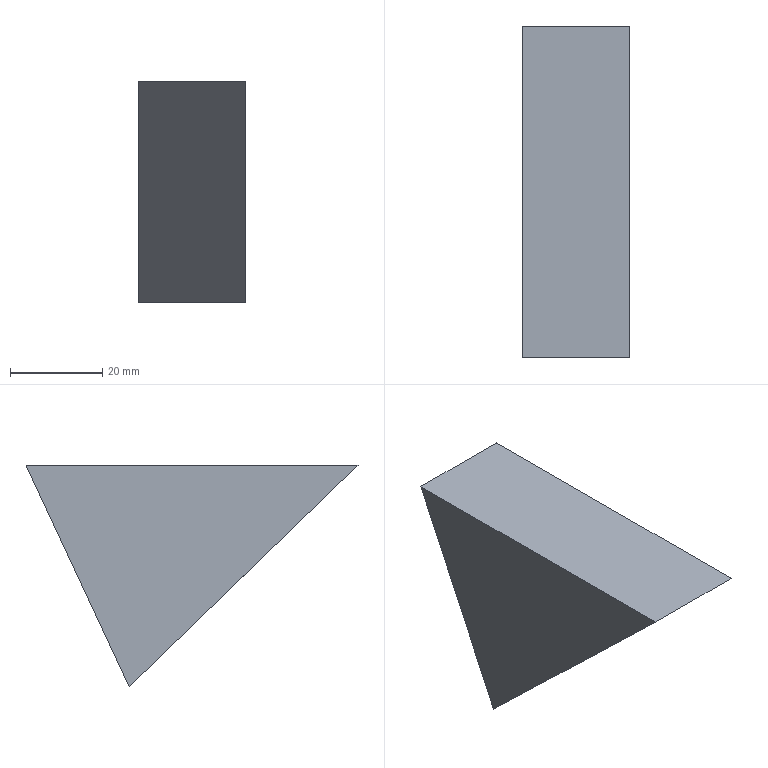Part | Creo | 1 solid | 5 faces | box 23.287 x 72.174 x 48.057 mm | volume 40385 mm3 | plane 5
STEP:
#1=CARTESIAN_POINT('',(0.,0.,0.));
#2=DIRECTION('',(0.,0.,1.));
#3=DIRECTION('',(1.,0.,0.));
#4=AXIS2_PLACEMENT_3D('',#1,#2,#3);
#5=CARTESIAN_POINT('',(-29.668,145.852,-81.892));
#6=VERTEX_POINT('',#5);
#7=CARTESIAN_POINT('',(-6.381,145.852,-81.892));
#8=VERTEX_POINT('',#7);
#9=CARTESIAN_POINT('',(-29.668,145.852,-81.892));
#10=DIRECTION('',(1.,0.000000105,-0.000000013));
#11=VECTOR('',#10,23.287);
#12=LINE('',#9,#11);
#13=EDGE_CURVE('',#6,#8,#12,.T.);
#14=ORIENTED_EDGE('',*,*,#13,.F.);
#15=CARTESIAN_POINT('',(-29.668,96.087,-33.835));
#16=VERTEX_POINT('',#15);
#17=CARTESIAN_POINT('',(-29.668,145.852,-81.892));
#18=DIRECTION('',(0.000000033,-0.7193,0.6947));
#19=VECTOR('',#18,69.181);
#20=LINE('',#17,#19);
#21=EDGE_CURVE('',#6,#16,#20,.T.);
#22=ORIENTED_EDGE('',*,*,#21,.T.);
#23=CARTESIAN_POINT('',(-6.381,96.087,-33.835));
#24=VERTEX_POINT('',#23);
#25=CARTESIAN_POINT('',(-6.381,96.087,-33.835));
#26=DIRECTION('',(-1.,-0.000000303,0.000000195));
#27=VECTOR('',#26,23.287);
#28=LINE('',#25,#27);
#29=EDGE_CURVE('',#24,#16,#28,.T.);
#30=ORIENTED_EDGE('',*,*,#29,.F.);
#31=CARTESIAN_POINT('',(-6.381,96.087,-33.835));
#32=DIRECTION('',(0.,0.7193,-0.6947));
#33=VECTOR('',#32,69.181);
#34=LINE('',#31,#33);
#35=EDGE_CURVE('',#24,#8,#34,.T.);
#36=ORIENTED_EDGE('',*,*,#35,.T.);
#37=EDGE_LOOP('',(#14,#22,#30,#36));
#38=FACE_OUTER_BOUND('',#37,.F.);
#39=CARTESIAN_POINT('',(-13.325,113.851,-50.989));
#40=DIRECTION('',(-0.000000063,0.6947,0.7193));
#41=DIRECTION('',(0.,-0.7193,0.6947));
#42=AXIS2_PLACEMENT_3D('',#39,#40,#41);
#43=PLANE('',#42);
#44=ADVANCED_FACE('',(#38),#43,.F.);
#45=CARTESIAN_POINT('',(-29.668,168.261,-33.835));
#46=VERTEX_POINT('',#45);
#47=CARTESIAN_POINT('',(-29.668,168.261,-33.835));
#48=DIRECTION('',(0.000000019,-0.4226,-0.9063));
#49=VECTOR('',#48,53.025);
#50=LINE('',#47,#49);
#51=EDGE_CURVE('',#46,#6,#50,.T.);
#52=ORIENTED_EDGE('',*,*,#51,.T.);
#53=ORIENTED_EDGE('',*,*,#13,.T.);
#54=CARTESIAN_POINT('',(-6.381,168.261,-33.835));
#55=VERTEX_POINT('',#54);
#56=CARTESIAN_POINT('',(-6.381,145.852,-81.892));
#57=DIRECTION('',(0.,0.4226,0.9063));
#58=VECTOR('',#57,53.025);
#59=LINE('',#56,#58);
#60=EDGE_CURVE('',#8,#55,#59,.T.);
#61=ORIENTED_EDGE('',*,*,#60,.T.);
#62=CARTESIAN_POINT('',(-6.381,168.261,-33.835));
#63=DIRECTION('',(-1.,-0.000000025,0.000000185));
#64=VECTOR('',#63,23.287);
#65=LINE('',#62,#64);
#66=EDGE_CURVE('',#55,#46,#65,.T.);
#67=ORIENTED_EDGE('',*,*,#66,.T.);
#68=EDGE_LOOP('',(#52,#53,#61,#67));
#69=FACE_OUTER_BOUND('',#68,.F.);
#70=CARTESIAN_POINT('',(-6.241,168.261,-33.835));
#71=DIRECTION('',(-0.000000101,0.9063,-0.4226));
#72=DIRECTION('',(0.,0.4226,0.9063));
#73=AXIS2_PLACEMENT_3D('',#70,#71,#72);
#74=PLANE('',#73);
#75=ADVANCED_FACE('',(#69),#74,.T.);
#76=ORIENTED_EDGE('',*,*,#21,.F.);
#77=ORIENTED_EDGE('',*,*,#51,.F.);
#78=CARTESIAN_POINT('',(-29.668,96.087,-33.835));
#79=DIRECTION('',(-0.000000046,1.,-0.000000009));
#80=VECTOR('',#79,72.174);
#81=LINE('',#78,#80);
#82=EDGE_CURVE('',#16,#46,#81,.T.);
#83=ORIENTED_EDGE('',*,*,#82,.F.);
#84=EDGE_LOOP('',(#76,#77,#83));
#85=FACE_OUTER_BOUND('',#84,.F.);
#86=CARTESIAN_POINT('',(-29.668,80.496,-15.998));
#87=DIRECTION('',(1.,0.000000046,0.));
#88=DIRECTION('',(-0.000000046,1.,0.));
#89=AXIS2_PLACEMENT_3D('',#86,#87,#88);
#90=PLANE('',#89);
#91=ADVANCED_FACE('',(#85),#90,.F.);
#92=ORIENTED_EDGE('',*,*,#82,.T.);
#93=ORIENTED_EDGE('',*,*,#66,.F.);
#94=CARTESIAN_POINT('',(-6.381,96.087,-33.835));
#95=DIRECTION('',(0.,1.,-0.000000006));
#96=VECTOR('',#95,72.174);
#97=LINE('',#94,#96);
#98=EDGE_CURVE('',#24,#55,#97,.T.);
#99=ORIENTED_EDGE('',*,*,#98,.F.);
#100=ORIENTED_EDGE('',*,*,#29,.T.);
#101=EDGE_LOOP('',(#92,#93,#99,#100));
#102=FACE_OUTER_BOUND('',#101,.F.);
#103=CARTESIAN_POINT('',(74.211,10000095.765,-33.835));
#104=DIRECTION('',(-0.000000175,0.,-1.));
#105=DIRECTION('',(-1.,0.,0.000000175));
#106=AXIS2_PLACEMENT_3D('',#103,#104,#105);
#107=PLANE('',#106);
#108=ADVANCED_FACE('',(#102),#107,.F.);
#109=ORIENTED_EDGE('',*,*,#60,.F.);
#110=ORIENTED_EDGE('',*,*,#35,.F.);
#111=ORIENTED_EDGE('',*,*,#98,.T.);
#112=EDGE_LOOP('',(#109,#110,#111));
#113=FACE_OUTER_BOUND('',#112,.F.);
#114=CARTESIAN_POINT('',(-6.381,101.276,-38.756));
#115=DIRECTION('',(1.,0.,0.));
#116=DIRECTION('',(0.,0.,-1.));
#117=AXIS2_PLACEMENT_3D('',#114,#115,#116);
#118=PLANE('',#117);
#119=ADVANCED_FACE('',(#113),#118,.T.);
#120=CLOSED_SHELL('',(#44,#75,#91,#108,#119));
#121=MANIFOLD_SOLID_BREP('',#120);
#122=(LENGTH_UNIT()NAMED_UNIT(*)SI_UNIT(.MILLI.,.METRE.));
#123=UNCERTAINTY_MEASURE_WITH_UNIT(LENGTH_MEASURE(0.008978),#122,'','');
#124=(NAMED_UNIT(*)PLANE_ANGLE_UNIT()SI_UNIT($,.RADIAN.));
#125=PLANE_ANGLE_MEASURE_WITH_UNIT(PLANE_ANGLE_MEASURE(0.01745),#124);
#126=(CONVERSION_BASED_UNIT('DEGREE',#125)NAMED_UNIT(*)PLANE_ANGLE_UNIT());
#127=(NAMED_UNIT(*)SI_UNIT($,.STERADIAN.)SOLID_ANGLE_UNIT());
#128=(GEOMETRIC_REPRESENTATION_CONTEXT(3)GLOBAL_UNCERTAINTY_ASSIGNED_CONTEXT((#123))GLOBAL_UNIT_ASSIGNED_CONTEXT((#122,#126,#127))REPRESENTATION_CONTEXT('',''));
#129=ADVANCED_BREP_SHAPE_REPRESENTATION('',(#4,#121),#128);